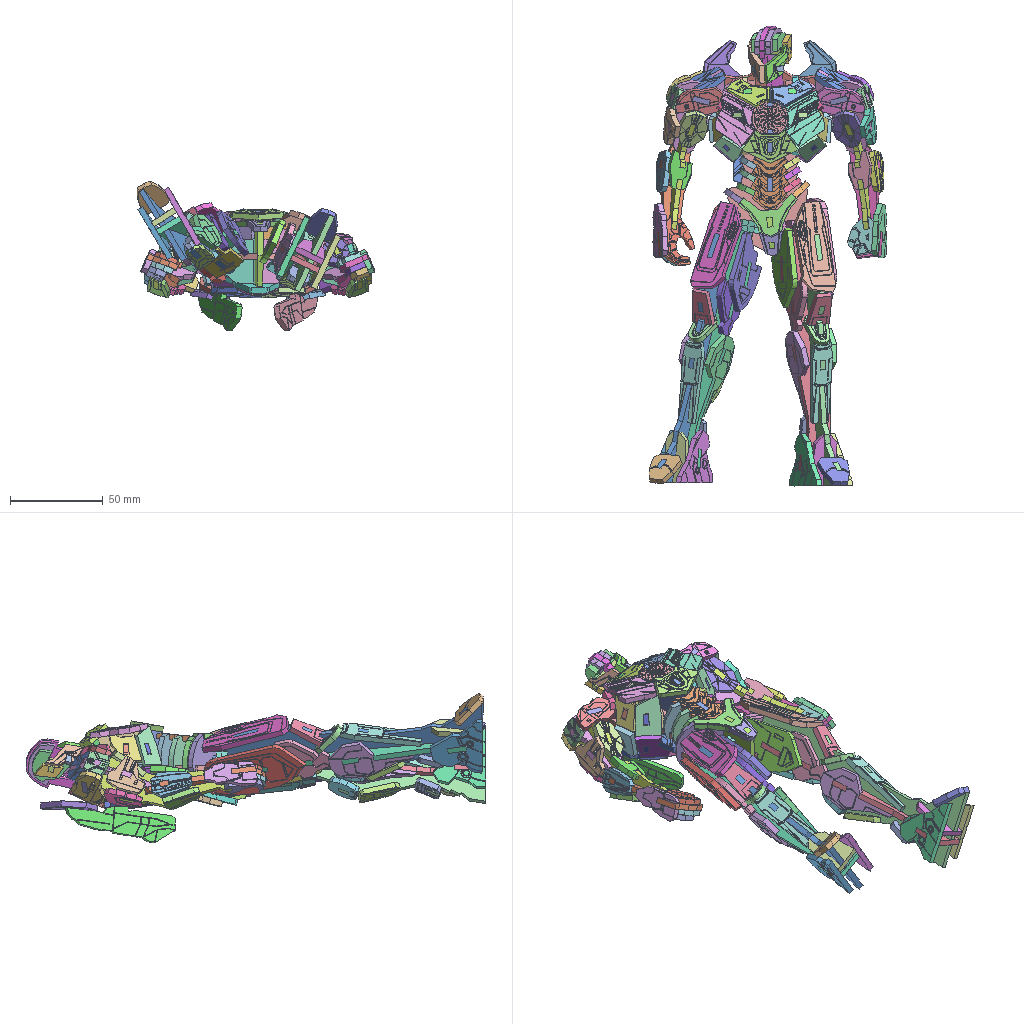Assembly | SolidWorks | 114 different items | 147 placed | box 128 x 248 x 81 mm
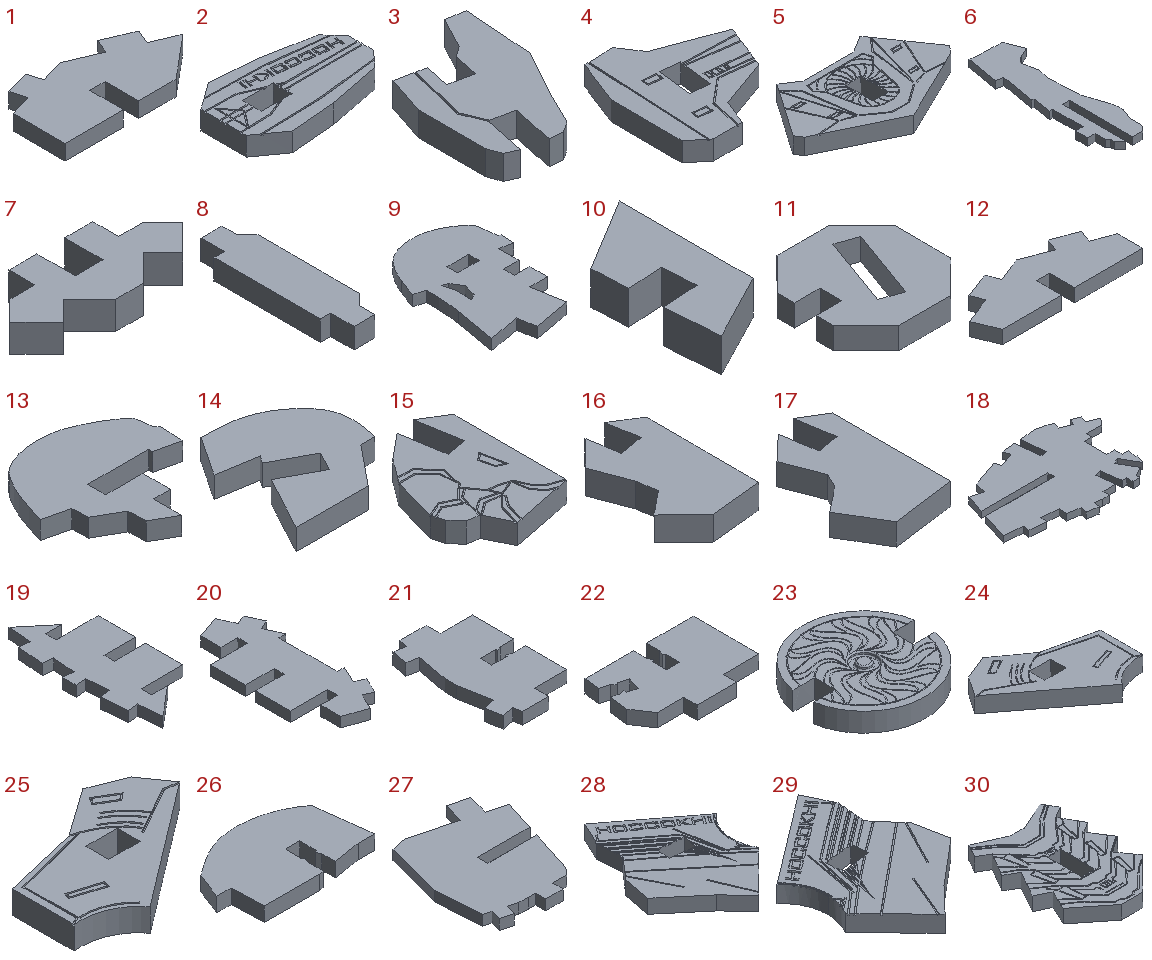Parts list (item | quantity | size | volume | features):
1 | x2 | 30.19 x 15.728 x 3 mm | 976.477 mm3 | features BaseBody 1
2 | x1 | 21.822 x 13.322 x 3 mm | 656.047 mm3 | features BaseBody 1
3 | x1 | 13.603 x 19.375 x 3 mm | 451.595 mm3 | features BaseBody 1
4 | x1 | 19.081 x 20.339 x 3 mm | 705.753 mm3 | features BaseBody 1
5 | x1 | 29.201 x 17.776 x 3 mm | 913.364 mm3 | features BaseBody 1
6 | x1 | 19.346 x 61.524 x 3 mm | 2044 mm3 | features BaseBody 1
7 | x1 | 18.567 x 8.438 x 3 mm | 257.816 mm3 | features BaseBody 1
8 | x1 | 6.137 x 22.551 x 3 mm | 356.006 mm3 | features BaseBody 1
9 | x1 | 27.077 x 39.16 x 3 mm | 2127 mm3 | features BaseBody 1
10 | x2 | 6.477 x 14.965 x 3 mm | 188.364 mm3 | features BaseBody 1
11 | x1 | 16.185 x 16.813 x 3 mm | 570.375 mm3 | features BaseBody 1
12 | x2 | 34.167 x 12.73 x 3 mm | 940.893 mm3 | features BaseBody 1
13 | x2 | 23.312 x 22.774 x 3 mm | 818.077 mm3 | features BaseBody 1
14 | x2 | 17.352 x 17.888 x 3 mm | 573.183 mm3 | features BaseBody 1
15 | x1 | 14.575 x 20.753 x 3 mm | 629.873 mm3 | features BaseBody 1
16 | x1 | 10.052 x 16.622 x 3 mm | 347.373 mm3 | features BaseBody 1
17 | x1 | 12.009 x 19.33 x 3 mm | 454.514 mm3 | features BaseBody 1
18 | x1 | 71.254 x 46.863 x 3 mm | 5844 mm3 | features BaseBody 1
19 | x1 | 20.269 x 43.799 x 3 mm | 1567 mm3 | features BaseBody 1
20 | x1 | 19.907 x 46.828 x 3 mm | 1794 mm3 | features BaseBody 1
21 | x1 | 19.083 x 31.429 x 3 mm | 1367 mm3 | features BaseBody 1
22 | x2 | 25.767 x 17.806 x 3 mm | 1076 mm3 | features BaseBody 1
23 | x1 | 19.154 x 19.434 x 3 mm | 813.614 mm3 | features BaseBody 1
24 | x1 | 23.095 x 17.792 x 3 mm | 604.555 mm3 | features BaseBody 1
25 | x1 | 23.105 x 17.792 x 3 mm | 604.662 mm3 | features BaseBody 1
26 | x1 | 27.839 x 17.276 x 3 mm | 1069 mm3 | features BaseBody 1
27 | x1 | 32.712 x 38.137 x 3 mm | 2525 mm3 | features BaseBody 1
28 | x1 | 23.207 x 32.146 x 3 mm | 1195 mm3 | features BaseBody 1
29 | x1 | 23.207 x 32.146 x 3 mm | 1195 mm3 | features BaseBody 1
30 | x1 | 20.837 x 28.283 x 3 mm | 1191 mm3 | features BaseBody 1
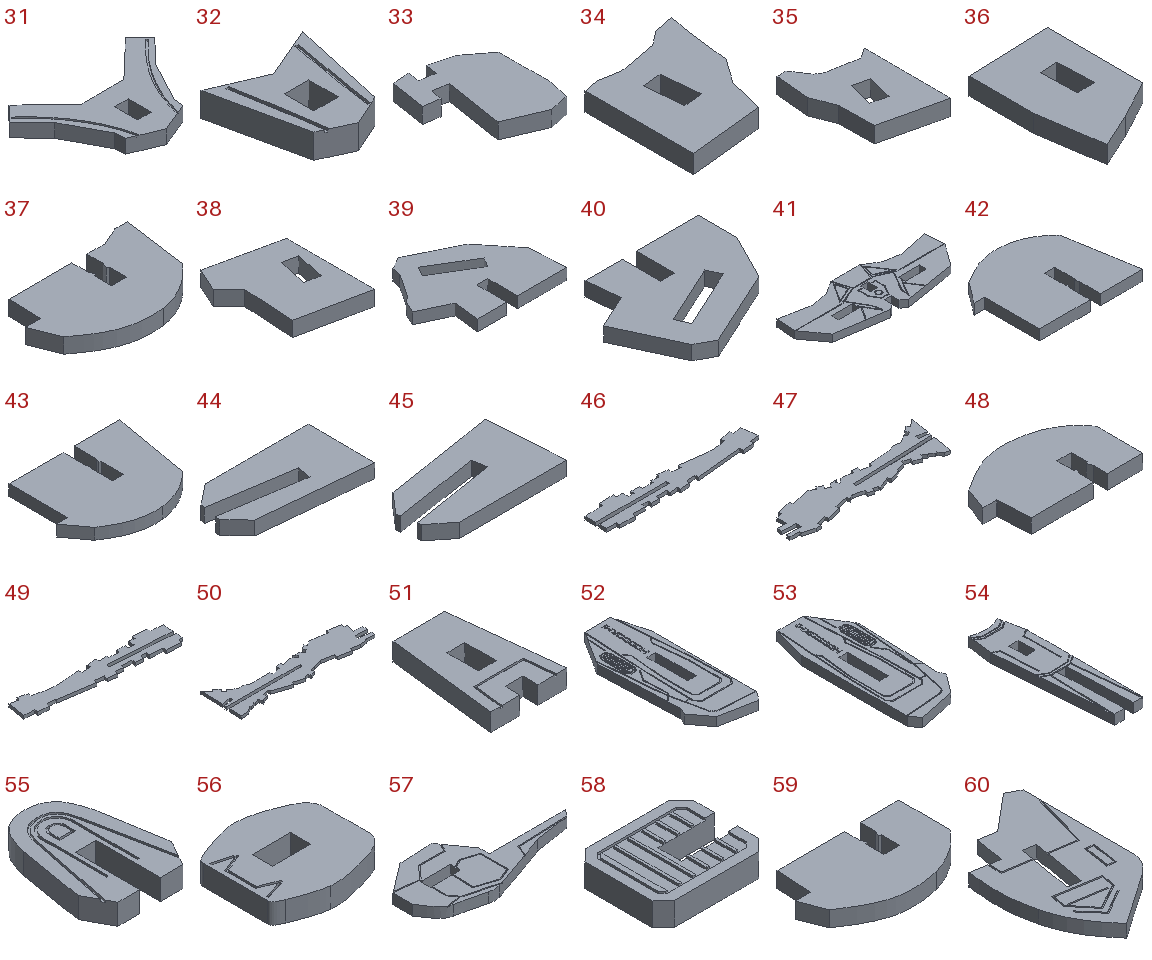31 | x1 | 31.951 x 21.72 x 3 mm | 821.926 mm3 | features BaseBody 1
32 | x1 | 12.536 x 13.11 x 3 mm | 276.053 mm3 | features BaseBody 1
33 | x2 | 16.417 x 19.898 x 3 mm | 620.666 mm3 | features BaseBody 1
34 | x2 | 17.508 x 21.063 x 3 mm | 743.607 mm3 | features BaseBody 1
35 | x2 | 13.422 x 20.055 x 3 mm | 525.703 mm3 | features BaseBody 1
36 | x2 | 14.02 x 22.667 x 3 mm | 747.582 mm3 | features BaseBody 1
37 | x1 | 28.291 x 18.638 x 3 mm | 1097 mm3 | features BaseBody 1
38 | x2 | 16.323 x 20.843 x 3 mm | 699.822 mm3 | features BaseBody 1
39 | x2 | 31.393 x 25.119 x 3 mm | 1380 mm3 | features BaseBody 1
40 | x2 | 30.485 x 25.117 x 3 mm | 1409 mm3 | features BaseBody 1
41 | x1 | 62.988 x 22.726 x 3 mm | 2983 mm3 | features BaseBody 1
42 | x1 | 32.694 x 25.985 x 3 mm | 1909 mm3 | features BaseBody 1
43 | x1 | 32.694 x 25.987 x 3 mm | 1909 mm3 | features BaseBody 1
44 | x1 | 27.749 x 14.503 x 3 mm | 877.652 mm3 | features BaseBody 1
45 | x1 | 28.09 x 16.288 x 3 mm | 953.359 mm3 | features BaseBody 1
46 | x1 | 140.807 x 26.276 x 3 mm | 6548 mm3 | features BaseBody 1
47 | x1 | 153.331 x 43.468 x 3 mm | 9745 mm3 | features BaseBody 1
48 | x1 | 26.661 x 16.081 x 3 mm | 988.736 mm3 | features BaseBody 1
49 | x1 | 137.742 x 31.731 x 3 mm | 6475 mm3 | features BaseBody 1
50 | x1 | 146.238 x 44.263 x 3 mm | 9488 mm3 | features BaseBody 1
51 | x2 | 12.712 x 18.351 x 3 mm | 516.696 mm3 | features BaseBody 1
52 | x1 | 18.994 x 49.692 x 3 mm | 2324 mm3 | features BaseBody 1
53 | x1 | 18.994 x 49.692 x 3 mm | 2324 mm3 | features BaseBody 1
54 | x2 | 11.853 x 44.2 x 3 mm | 1124 mm3 | features BaseBody 1
55 | x2 | 13.412 x 18.194 x 3 mm | 493.747 mm3 | features BaseBody 1
56 | x2 | 16.136 x 15.14 x 3 mm | 585.362 mm3 | features BaseBody 1
57 | x2 | 46.751 x 20.92 x 3 mm | 1382 mm3 | features BaseBody 1
58 | x2 | 13.855 x 11.523 x 3 mm | 379.654 mm3 | features BaseBody 1
59 | x1 | 26.677 x 16.089 x 3 mm | 988.858 mm3 | features BaseBody 1
60 | x1 | 23.87 x 41.361 x 3 mm | 1927 mm3 | features BaseBody 1
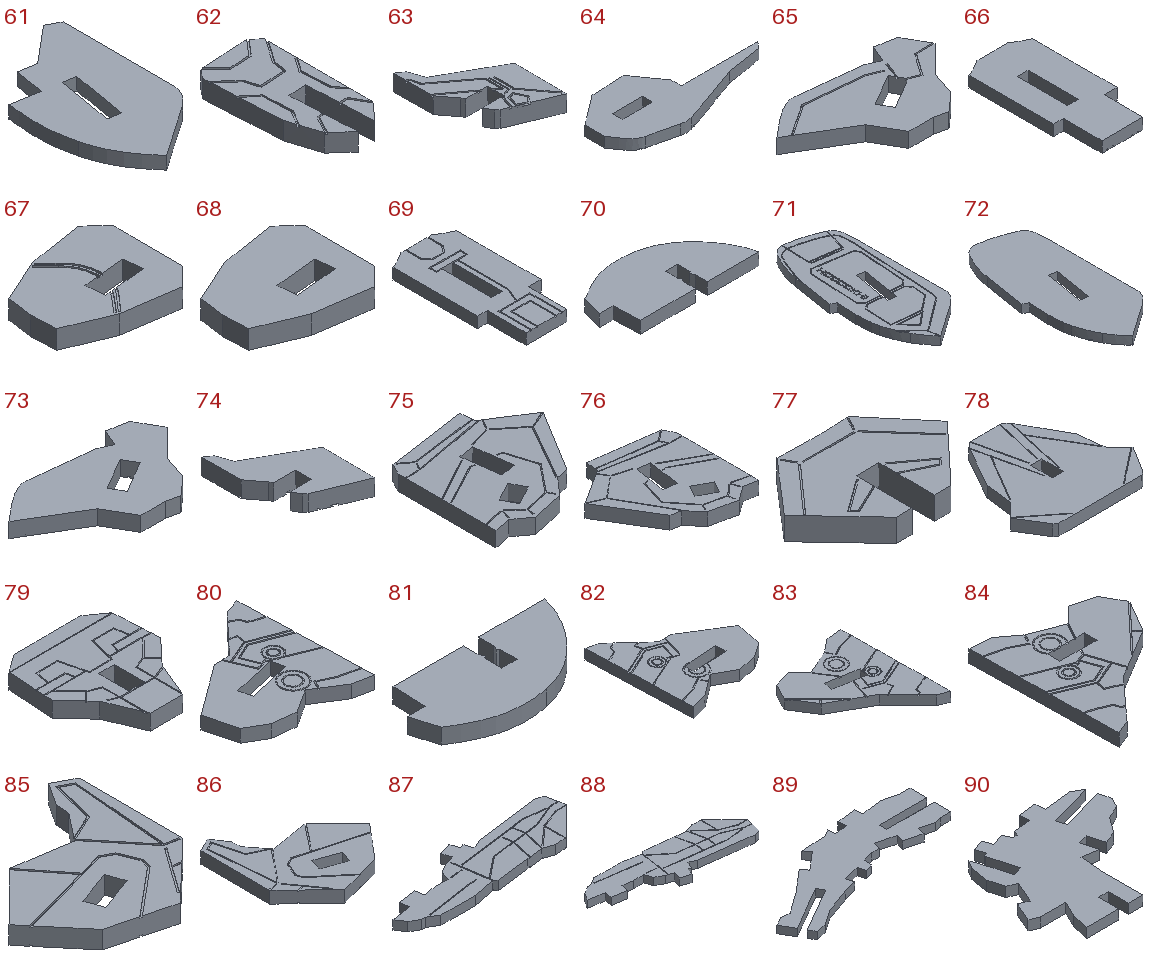61 | x1 | 23.87 x 41.361 x 3 mm | 1927 mm3 | features BaseBody 1
62 | x2 | 10.99 x 22.898 x 3 mm | 554.392 mm3 | features BaseBody 1
63 | x1 | 12.769 x 19.344 x 3 mm | 333.771 mm3 | features BaseBody 1
64 | x2 | 46.751 x 20.92 x 3 mm | 1382 mm3 | features BaseBody 1
65 | x2 | 32.789 x 19.083 x 3 mm | 1028 mm3 | features BaseBody 1
66 | x1 | 17.454 x 36.156 x 3 mm | 1527 mm3 | features BaseBody 1
67 | x1 | 19 x 16.741 x 3 mm | 696.97 mm3 | features BaseBody 1
68 | x1 | 19 x 16.741 x 3 mm | 696.97 mm3 | features BaseBody 1
69 | x1 | 17.454 x 36.156 x 3 mm | 1527 mm3 | features BaseBody 1
70 | x1 | 33.145 x 15.784 x 3 mm | 1116 mm3 | features BaseBody 1
71 | x1 | 25.301 x 57.359 x 3 mm | 3340 mm3 | features BaseBody 1
72 | x1 | 25.301 x 57.359 x 3 mm | 3340 mm3 | features BaseBody 1
73 | x2 | 32.789 x 19.083 x 3 mm | 1028 mm3 | features BaseBody 1
74 | x1 | 12.769 x 19.344 x 3 mm | 333.771 mm3 | features BaseBody 1
75 | x1 | 25.081 x 25.399 x 3 mm | 1254 mm3 | features BaseBody 1
76 | x1 | 25.081 x 25.399 x 3 mm | 1254 mm3 | features BaseBody 1
77 | x1 | 21.443 x 14.616 x 3 mm | 580.976 mm3 | features BaseBody 1
78 | x1 | 32.817 x 30.753 x 3 mm | 2054 mm3 | features BaseBody 1
79 | x1 | 20.921 x 23.01 x 3 mm | 1032 mm3 | features BaseBody 1
80 | x1 | 28.584 x 31.242 x 3 mm | 1486 mm3 | features BaseBody 1
81 | x1 | 33.145 x 15.78 x 3 mm | 1115 mm3 | features BaseBody 1
82 | x1 | 28.758 x 31.242 x 3 mm | 1487 mm3 | features BaseBody 1
83 | x1 | 28.805 x 34.776 x 3 mm | 1576 mm3 | features BaseBody 1
84 | x1 | 28.565 x 34.776 x 3 mm | 1588 mm3 | features BaseBody 1
85 | x1 | 27.356 x 28.569 x 3 mm | 1227 mm3 | features BaseBody 1
86 | x1 | 27.356 x 28.569 x 3 mm | 1227 mm3 | features BaseBody 1
87 | x1 | 62.766 x 19.221 x 3 mm | 2190 mm3 | features BaseBody 1
88 | x1 | 62.766 x 19.221 x 3 mm | 2190 mm3 | features BaseBody 1
89 | x2 | 75.297 x 35.268 x 3 mm | 3149 mm3 | features BaseBody 1
90 | x2 | 45.454 x 40.899 x 3 mm | 2775 mm3 | features BaseBody 1
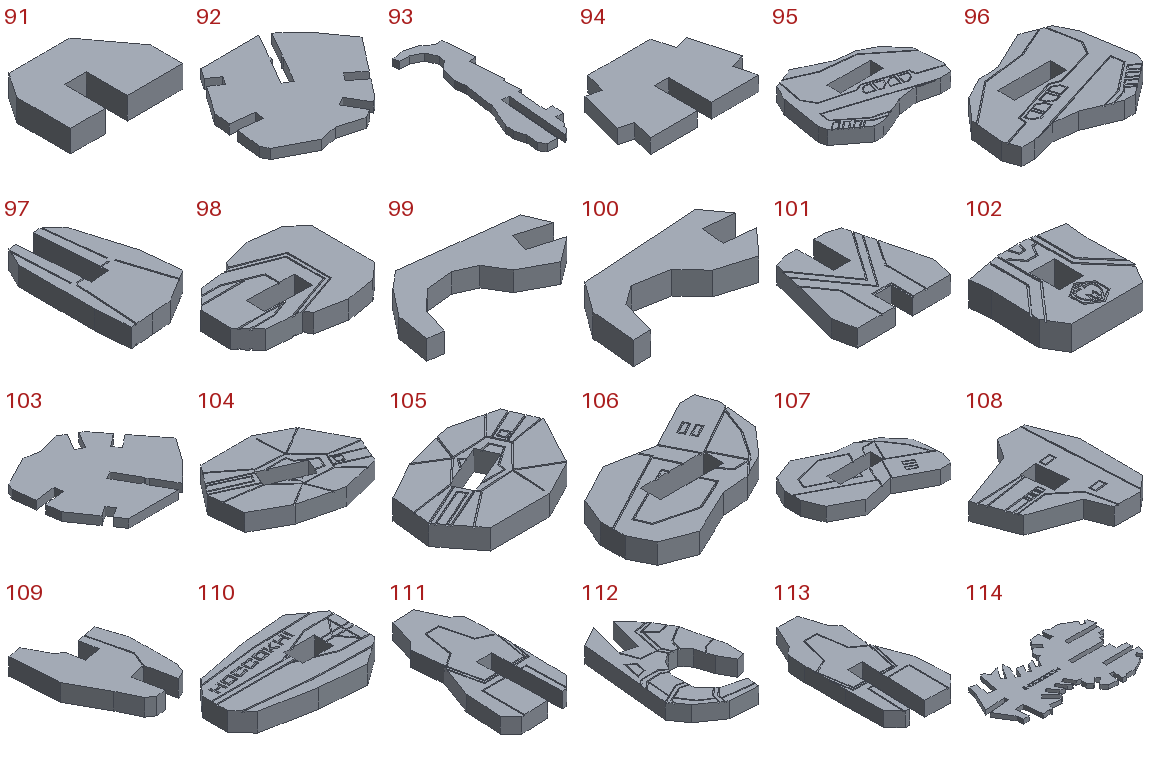91 | x2 | 15.248 x 10.684 x 3 mm | 381.769 mm3 | features BaseBody 1
92 | x1 | 45.246 x 38.746 x 3 mm | 3417 mm3 | features BaseBody 1
93 | x1 | 19.065 x 65.26 x 3 mm | 1941 mm3 | features BaseBody 1
94 | x2 | 25.93 x 17.686 x 3 mm | 1031 mm3 | features BaseBody 1
95 | x1 | 25.647 x 19.802 x 3 mm | 997.397 mm3 | features BaseBody 1
96 | x1 | 25.647 x 19.802 x 3 mm | 997.397 mm3 | features BaseBody 1
97 | x2 | 12.359 x 20.834 x 3 mm | 528.554 mm3 | features BaseBody 1
98 | x2 | 20.777 x 16.014 x 3 mm | 719.553 mm3 | features BaseBody 1
99 | x1 | 25.116 x 11.758 x 3 mm | 409.356 mm3 | features BaseBody 1
100 | x1 | 20.938 x 10.659 x 3 mm | 345.483 mm3 | features BaseBody 1
101 | x4 | 17.999 x 17.317 x 3 mm | 684.94 mm3 | features BaseBody 1
102 | x2 | 11.849 x 11.702 x 3 mm | 350.145 mm3 | features BaseBody 1
103 | x1 | 45.246 x 38.744 x 3 mm | 3417 mm3 | features BaseBody 1
104 | x1 | 21.888 x 16.021 x 3 mm | 729.931 mm3 | features BaseBody 1
105 | x1 | 21.888 x 16.021 x 3 mm | 729.931 mm3 | features BaseBody 1
106 | x1 | 24.24 x 17.887 x 3 mm | 761.054 mm3 | features BaseBody 1
107 | x1 | 24.24 x 17.887 x 3 mm | 761.054 mm3 | features BaseBody 1
108 | x1 | 19.081 x 20.339 x 3 mm | 705.753 mm3 | features BaseBody 1
109 | x1 | 13.603 x 19.375 x 3 mm | 451.595 mm3 | features BaseBody 1
110 | x1 | 21.822 x 13.322 x 3 mm | 656.047 mm3 | features BaseBody 1
111 | x1 | 13.49 x 28.35 x 3 mm | 780.38 mm3 | features BaseBody 1
112 | x1 | 15.584 x 25.481 x 3 mm | 593.723 mm3 | features BaseBody 1
113 | x1 | 13.49 x 28.35 x 3 mm | 780.38 mm3 | features BaseBody 1
114 | x1 | 94.912 x 58.414 x 3 mm | 9467 mm3 | features BaseBody 1